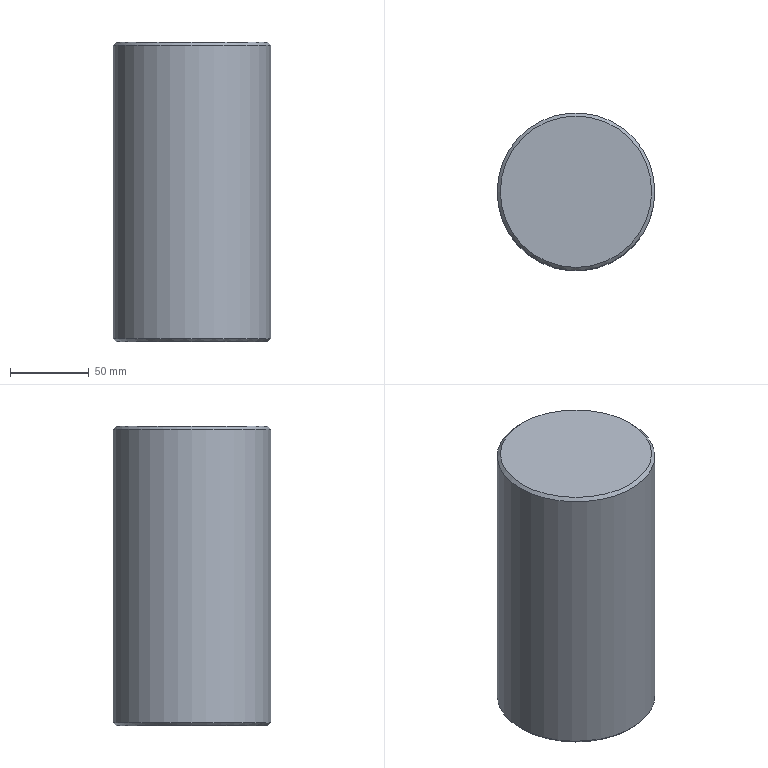Part | STEP file | lll_id854_x_t | 1 solid | 7 faces | box 100 x 100 x 190 mm | volume 1484379 mm3 | cone 3 | plane 2 | cylinder 2 | commonest cylinder face diameters 14.505 x1 100 x1
STEP:
#1=CARTESIAN_POINT('',(3144.435,-507.879,-370.));
#2=VERTEX_POINT('',#1);
#3=CARTESIAN_POINT('',(3192.435,-507.879,-370.));
#4=DIRECTION('',(0.,0.,-1.));
#5=DIRECTION('',(-1.,0.,0.));
#6=AXIS2_PLACEMENT_3D('',#3,#4,#5);
#7=CIRCLE('',#6,48.);
#8=EDGE_CURVE('',#2,#2,#7,.T.);
#9=ORIENTED_EDGE('',*,*,#8,.T.);
#10=EDGE_LOOP('',(#9));
#11=FACE_BOUND('',#10,.T.);
#12=CARTESIAN_POINT('',(3199.688,-507.879,-370.));
#13=VERTEX_POINT('',#12);
#14=CARTESIAN_POINT('',(3192.435,-507.879,-370.));
#15=DIRECTION('',(0.,0.,1.));
#16=DIRECTION('',(1.,0.,0.));
#17=AXIS2_PLACEMENT_3D('',#14,#15,#16);
#18=CIRCLE('',#17,7.253);
#19=EDGE_CURVE('',#13,#13,#18,.T.);
#20=ORIENTED_EDGE('',*,*,#19,.T.);
#21=EDGE_LOOP('',(#20));
#22=FACE_BOUND('',#21,.T.);
#23=CARTESIAN_POINT('',(3192.435,-507.879,-370.));
#24=DIRECTION('',(0.,0.,-1.));
#25=DIRECTION('',(1.,0.,0.));
#26=AXIS2_PLACEMENT_3D('',#23,#24,#25);
#27=PLANE('',#26);
#28=ADVANCED_FACE('',(#11,#22),#27,.T.);
#29=CARTESIAN_POINT('',(3240.435,-507.879,-180.));
#30=VERTEX_POINT('',#29);
#31=CARTESIAN_POINT('',(3192.435,-507.879,-180.));
#32=DIRECTION('',(0.,0.,1.));
#33=DIRECTION('',(1.,0.,0.));
#34=AXIS2_PLACEMENT_3D('',#31,#32,#33);
#35=CIRCLE('',#34,48.);
#36=EDGE_CURVE('',#30,#30,#35,.T.);
#37=ORIENTED_EDGE('',*,*,#36,.T.);
#38=EDGE_LOOP('',(#37));
#39=FACE_OUTER_BOUND('',#38,.T.);
#40=CARTESIAN_POINT('',(3192.435,-507.879,-180.));
#41=DIRECTION('',(0.,0.,1.));
#42=DIRECTION('',(-1.,0.,0.));
#43=AXIS2_PLACEMENT_3D('',#40,#41,#42);
#44=PLANE('',#43);
#45=ADVANCED_FACE('',(#39),#44,.T.);
#46=CARTESIAN_POINT('',(3142.435,-507.879,-182.));
#47=VERTEX_POINT('',#46);
#48=CARTESIAN_POINT('',(3192.435,-507.879,-182.));
#49=DIRECTION('',(0.,0.,-1.));
#50=DIRECTION('',(-1.,0.,0.));
#51=AXIS2_PLACEMENT_3D('',#48,#49,#50);
#52=CIRCLE('',#51,50.);
#53=EDGE_CURVE('',#47,#47,#52,.T.);
#54=ORIENTED_EDGE('',*,*,#53,.T.);
#55=EDGE_LOOP('',(#54));
#56=FACE_BOUND('',#55,.T.);
#57=CARTESIAN_POINT('',(3242.435,-507.879,-368.));
#58=VERTEX_POINT('',#57);
#59=CARTESIAN_POINT('',(3192.435,-507.879,-368.));
#60=DIRECTION('',(0.,0.,1.));
#61=DIRECTION('',(1.,0.,0.));
#62=AXIS2_PLACEMENT_3D('',#59,#60,#61);
#63=CIRCLE('',#62,50.);
#64=EDGE_CURVE('',#58,#58,#63,.T.);
#65=ORIENTED_EDGE('',*,*,#64,.T.);
#66=EDGE_LOOP('',(#65));
#67=FACE_BOUND('',#66,.T.);
#68=CARTESIAN_POINT('',(3192.435,-507.879,-180.));
#69=DIRECTION('',(0.,0.,-1.));
#70=DIRECTION('',(1.,0.,0.));
#71=AXIS2_PLACEMENT_3D('',#68,#69,#70);
#72=CYLINDRICAL_SURFACE('',#71,50.);
#73=ADVANCED_FACE('',(#56,#67),#72,.T.);
#74=ORIENTED_EDGE('',*,*,#36,.F.);
#75=EDGE_LOOP('',(#74));
#76=FACE_BOUND('',#75,.T.);
#77=ORIENTED_EDGE('',*,*,#53,.F.);
#78=EDGE_LOOP('',(#77));
#79=FACE_BOUND('',#78,.T.);
#80=CARTESIAN_POINT('',(3192.435,-507.879,-182.));
#81=DIRECTION('',(0.,0.,-1.));
#82=DIRECTION('',(1.,0.,0.));
#83=AXIS2_PLACEMENT_3D('',#80,#81,#82);
#84=CONICAL_SURFACE('',#83,50.,45.);
#85=ADVANCED_FACE('',(#76,#79),#84,.T.);
#86=ORIENTED_EDGE('',*,*,#8,.F.);
#87=EDGE_LOOP('',(#86));
#88=FACE_BOUND('',#87,.T.);
#89=ORIENTED_EDGE('',*,*,#64,.F.);
#90=EDGE_LOOP('',(#89));
#91=FACE_BOUND('',#90,.T.);
#92=CARTESIAN_POINT('',(3192.435,-507.879,-368.));
#93=DIRECTION('',(0.,0.,1.));
#94=DIRECTION('',(-1.,0.,0.));
#95=AXIS2_PLACEMENT_3D('',#92,#93,#94);
#96=CONICAL_SURFACE('',#95,50.,45.);
#97=ADVANCED_FACE('',(#88,#91),#96,.T.);
#98=CARTESIAN_POINT('',(3199.688,-507.879,-332.247));
#99=VERTEX_POINT('',#98);
#100=CARTESIAN_POINT('',(3192.435,-507.879,-332.247));
#101=DIRECTION('',(0.,0.,1.));
#102=DIRECTION('',(1.,0.,0.));
#103=AXIS2_PLACEMENT_3D('',#100,#101,#102);
#104=CIRCLE('',#103,7.253);
#105=EDGE_CURVE('',#99,#99,#104,.T.);
#106=ORIENTED_EDGE('',*,*,#105,.T.);
#107=EDGE_LOOP('',(#106));
#108=FACE_BOUND('',#107,.T.);
#109=ORIENTED_EDGE('',*,*,#19,.F.);
#110=EDGE_LOOP('',(#109));
#111=FACE_BOUND('',#110,.T.);
#112=CARTESIAN_POINT('',(3192.435,-507.879,-370.));
#113=DIRECTION('',(0.,0.,1.));
#114=DIRECTION('',(-1.,0.,0.));
#115=AXIS2_PLACEMENT_3D('',#112,#113,#114);
#116=CYLINDRICAL_SURFACE('',#115,7.253);
#117=ADVANCED_FACE('',(#108,#111),#116,.F.);
#118=CARTESIAN_POINT('',(3192.435,-507.879,-324.994));
#119=VERTEX_POINT('',#118);
#120=VERTEX_LOOP('',#119);
#121=FACE_BOUND('',#120,.T.);
#122=ORIENTED_EDGE('',*,*,#105,.F.);
#123=EDGE_LOOP('',(#122));
#124=FACE_BOUND('',#123,.T.);
#125=CARTESIAN_POINT('',(3192.435,-507.879,-332.247));
#126=DIRECTION('',(0.,0.,-1.));
#127=DIRECTION('',(1.,0.,0.));
#128=AXIS2_PLACEMENT_3D('',#125,#126,#127);
#129=CONICAL_SURFACE('',#128,7.253,45.);
#130=ADVANCED_FACE('',(#121,#124),#129,.F.);
#131=CLOSED_SHELL('',(#28,#45,#73,#85,#97,#117,#130));
#132=MANIFOLD_SOLID_BREP('',#131);
#133=(LENGTH_UNIT()NAMED_UNIT(*)SI_UNIT(.MILLI.,.METRE.));
#134=UNCERTAINTY_MEASURE_WITH_UNIT(LENGTH_MEASURE(0.00002),#133,'','');
#135=(NAMED_UNIT(*)PLANE_ANGLE_UNIT()SI_UNIT($,.RADIAN.));
#136=PLANE_ANGLE_MEASURE_WITH_UNIT(PLANE_ANGLE_MEASURE(0.01745),#135);
#137=DIMENSIONAL_EXPONENTS(0.,0.,0.,0.,0.,0.,0.);
#138=(CONVERSION_BASED_UNIT('DEGREE',#136)NAMED_UNIT(#137)PLANE_ANGLE_UNIT());
#139=(NAMED_UNIT(*)SI_UNIT($,.STERADIAN.)SOLID_ANGLE_UNIT());
#140=(GEOMETRIC_REPRESENTATION_CONTEXT(3)GLOBAL_UNCERTAINTY_ASSIGNED_CONTEXT((#134))GLOBAL_UNIT_ASSIGNED_CONTEXT((#133,#138,#139))REPRESENTATION_CONTEXT('',''));
#141=ADVANCED_BREP_SHAPE_REPRESENTATION('',(#132),#140);